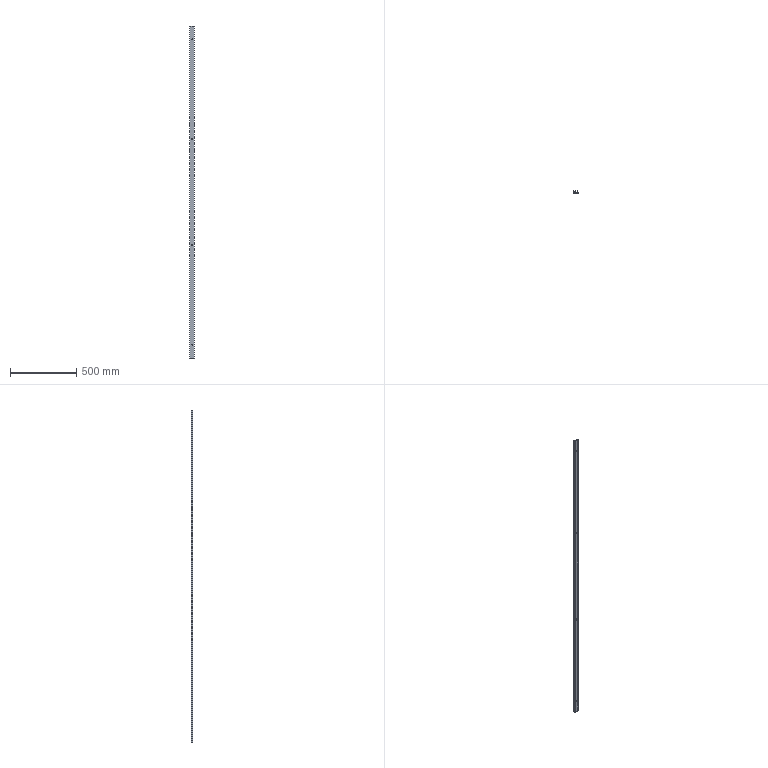Part | SolidWorks | features ICE 2, BaseBody 1, HoleWzd 1, MoveFace 1 | 1 solid | 35 faces | box 33.5 x 13.5 x 2500 mm | volume 468220 mm3 | plane 17 | cylinder 10 | cone 8 | commonest cylinder face diameters 13.44 x4 2 x3 4 x2 1.5 x1
STEP:
#1=CARTESIAN_POINT('',(20.,0.,2303.72));
#2=VERTEX_POINT('',#1);
#3=CARTESIAN_POINT('',(20.,0.,2296.28));
#4=VERTEX_POINT('',#3);
#5=CARTESIAN_POINT('',(20.,0.,2300.));
#6=DIRECTION('',(0.,-1.,0.));
#7=DIRECTION('',(0.,0.,-1.));
#8=AXIS2_PLACEMENT_3D('',#5,#6,#7);
#9=CIRCLE('',#8,3.72);
#10=EDGE_CURVE('',#2,#4,#9,.T.);
#11=ORIENTED_EDGE('',*,*,#10,.T.);
#12=CARTESIAN_POINT('',(20.,3.,2293.28));
#13=VERTEX_POINT('',#12);
#14=CARTESIAN_POINT('',(20.,3.,2293.28));
#15=DIRECTION('',(0.,0.7071,-0.7071));
#16=VECTOR('',#15,1000.);
#17=LINE('',#14,#16);
#18=EDGE_CURVE('',#4,#13,#17,.T.);
#19=ORIENTED_EDGE('',*,*,#18,.T.);
#20=CARTESIAN_POINT('',(20.,3.,2306.72));
#21=VERTEX_POINT('',#20);
#22=CARTESIAN_POINT('',(20.,3.,2300.));
#23=DIRECTION('',(0.,1.,0.));
#24=DIRECTION('',(0.,0.,1.));
#25=AXIS2_PLACEMENT_3D('',#22,#23,#24);
#26=CIRCLE('',#25,6.72);
#27=EDGE_CURVE('',#13,#21,#26,.T.);
#28=ORIENTED_EDGE('',*,*,#27,.T.);
#29=CARTESIAN_POINT('',(20.,3.,2306.72));
#30=DIRECTION('',(0.,0.7071,0.7071));
#31=VECTOR('',#30,1000.);
#32=LINE('',#29,#31);
#33=EDGE_CURVE('',#2,#21,#32,.T.);
#34=ORIENTED_EDGE('',*,*,#33,.F.);
#35=EDGE_LOOP('',(#11,#19,#28,#34));
#36=FACE_OUTER_BOUND('',#35,.T.);
#37=CARTESIAN_POINT('',(20.,3.,2300.));
#38=DIRECTION('',(0.,1.,0.));
#39=DIRECTION('',(0.,0.,1.));
#40=AXIS2_PLACEMENT_3D('',#37,#38,#39);
#41=CONICAL_SURFACE('',#40,6.72,0.7854);
#42=ADVANCED_FACE('',(#36),#41,.F.);
#43=CARTESIAN_POINT('',(20.,0.,3.72));
#44=VERTEX_POINT('',#43);
#45=CARTESIAN_POINT('',(20.,0.,-3.72));
#46=VERTEX_POINT('',#45);
#47=CARTESIAN_POINT('',(20.,0.,0.));
#48=DIRECTION('',(0.,-1.,0.));
#49=DIRECTION('',(0.,0.,-1.));
#50=AXIS2_PLACEMENT_3D('',#47,#48,#49);
#51=CIRCLE('',#50,3.72);
#52=EDGE_CURVE('',#44,#46,#51,.T.);
#53=ORIENTED_EDGE('',*,*,#52,.T.);
#54=CARTESIAN_POINT('',(20.,3.,-6.72));
#55=VERTEX_POINT('',#54);
#56=CARTESIAN_POINT('',(20.,3.,-6.72));
#57=DIRECTION('',(0.,0.7071,-0.7071));
#58=VECTOR('',#57,1000.);
#59=LINE('',#56,#58);
#60=EDGE_CURVE('',#46,#55,#59,.T.);
#61=ORIENTED_EDGE('',*,*,#60,.T.);
#62=CARTESIAN_POINT('',(20.,3.,6.72));
#63=VERTEX_POINT('',#62);
#64=CARTESIAN_POINT('',(20.,3.,0.));
#65=DIRECTION('',(0.,1.,0.));
#66=DIRECTION('',(0.,0.,1.));
#67=AXIS2_PLACEMENT_3D('',#64,#65,#66);
#68=CIRCLE('',#67,6.72);
#69=EDGE_CURVE('',#55,#63,#68,.T.);
#70=ORIENTED_EDGE('',*,*,#69,.T.);
#71=CARTESIAN_POINT('',(20.,3.,6.72));
#72=DIRECTION('',(0.,0.7071,0.7071));
#73=VECTOR('',#72,1000.);
#74=LINE('',#71,#73);
#75=EDGE_CURVE('',#44,#63,#74,.T.);
#76=ORIENTED_EDGE('',*,*,#75,.F.);
#77=EDGE_LOOP('',(#53,#61,#70,#76));
#78=FACE_OUTER_BOUND('',#77,.T.);
#79=CARTESIAN_POINT('',(20.,3.,0.));
#80=DIRECTION('',(0.,1.,0.));
#81=DIRECTION('',(0.,0.,1.));
#82=AXIS2_PLACEMENT_3D('',#79,#80,#81);
#83=CONICAL_SURFACE('',#82,6.72,0.7854);
#84=ADVANCED_FACE('',(#78),#83,.F.);
#85=CARTESIAN_POINT('',(20.,0.,753.72));
#86=VERTEX_POINT('',#85);
#87=CARTESIAN_POINT('',(20.,0.,746.28));
#88=VERTEX_POINT('',#87);
#89=CARTESIAN_POINT('',(20.,0.,750.));
#90=DIRECTION('',(0.,-1.,0.));
#91=DIRECTION('',(0.,0.,-1.));
#92=AXIS2_PLACEMENT_3D('',#89,#90,#91);
#93=CIRCLE('',#92,3.72);
#94=EDGE_CURVE('',#86,#88,#93,.T.);
#95=ORIENTED_EDGE('',*,*,#94,.T.);
#96=CARTESIAN_POINT('',(20.,3.,743.28));
#97=VERTEX_POINT('',#96);
#98=CARTESIAN_POINT('',(20.,3.,743.28));
#99=DIRECTION('',(0.,0.7071,-0.7071));
#100=VECTOR('',#99,1000.);
#101=LINE('',#98,#100);
#102=EDGE_CURVE('',#88,#97,#101,.T.);
#103=ORIENTED_EDGE('',*,*,#102,.T.);
#104=CARTESIAN_POINT('',(20.,3.,756.72));
#105=VERTEX_POINT('',#104);
#106=CARTESIAN_POINT('',(20.,3.,750.));
#107=DIRECTION('',(0.,1.,0.));
#108=DIRECTION('',(0.,0.,1.));
#109=AXIS2_PLACEMENT_3D('',#106,#107,#108);
#110=CIRCLE('',#109,6.72);
#111=EDGE_CURVE('',#97,#105,#110,.T.);
#112=ORIENTED_EDGE('',*,*,#111,.T.);
#113=CARTESIAN_POINT('',(20.,3.,756.72));
#114=DIRECTION('',(0.,0.7071,0.7071));
#115=VECTOR('',#114,1000.);
#116=LINE('',#113,#115);
#117=EDGE_CURVE('',#86,#105,#116,.T.);
#118=ORIENTED_EDGE('',*,*,#117,.F.);
#119=EDGE_LOOP('',(#95,#103,#112,#118));
#120=FACE_OUTER_BOUND('',#119,.T.);
#121=CARTESIAN_POINT('',(20.,3.,750.));
#122=DIRECTION('',(0.,1.,0.));
#123=DIRECTION('',(0.,0.,1.));
#124=AXIS2_PLACEMENT_3D('',#121,#122,#123);
#125=CONICAL_SURFACE('',#124,6.72,0.7854);
#126=ADVANCED_FACE('',(#120),#125,.F.);
#127=CARTESIAN_POINT('',(20.,0.,1553.72));
#128=VERTEX_POINT('',#127);
#129=CARTESIAN_POINT('',(20.,0.,1546.28));
#130=VERTEX_POINT('',#129);
#131=CARTESIAN_POINT('',(20.,0.,1550.));
#132=DIRECTION('',(0.,-1.,0.));
#133=DIRECTION('',(0.,0.,-1.));
#134=AXIS2_PLACEMENT_3D('',#131,#132,#133);
#135=CIRCLE('',#134,3.72);
#136=EDGE_CURVE('',#128,#130,#135,.T.);
#137=ORIENTED_EDGE('',*,*,#136,.T.);
#138=CARTESIAN_POINT('',(20.,3.,1543.28));
#139=VERTEX_POINT('',#138);
#140=CARTESIAN_POINT('',(20.,3.,1543.28));
#141=DIRECTION('',(0.,0.7071,-0.7071));
#142=VECTOR('',#141,1000.);
#143=LINE('',#140,#142);
#144=EDGE_CURVE('',#130,#139,#143,.T.);
#145=ORIENTED_EDGE('',*,*,#144,.T.);
#146=CARTESIAN_POINT('',(20.,3.,1556.72));
#147=VERTEX_POINT('',#146);
#148=CARTESIAN_POINT('',(20.,3.,1550.));
#149=DIRECTION('',(0.,1.,0.));
#150=DIRECTION('',(0.,0.,1.));
#151=AXIS2_PLACEMENT_3D('',#148,#149,#150);
#152=CIRCLE('',#151,6.72);
#153=EDGE_CURVE('',#139,#147,#152,.T.);
#154=ORIENTED_EDGE('',*,*,#153,.T.);
#155=CARTESIAN_POINT('',(20.,3.,1556.72));
#156=DIRECTION('',(0.,0.7071,0.7071));
#157=VECTOR('',#156,1000.);
#158=LINE('',#155,#157);
#159=EDGE_CURVE('',#128,#147,#158,.T.);
#160=ORIENTED_EDGE('',*,*,#159,.F.);
#161=EDGE_LOOP('',(#137,#145,#154,#160));
#162=FACE_OUTER_BOUND('',#161,.T.);
#163=CARTESIAN_POINT('',(20.,3.,1550.));
#164=DIRECTION('',(0.,1.,0.));
#165=DIRECTION('',(0.,0.,1.));
#166=AXIS2_PLACEMENT_3D('',#163,#164,#165);
#167=CONICAL_SURFACE('',#166,6.72,0.7854);
#168=ADVANCED_FACE('',(#162),#167,.F.);
#169=CARTESIAN_POINT('',(24.5,10.5,1545.009));
#170=VERTEX_POINT('',#169);
#171=CARTESIAN_POINT('',(24.5,10.5,754.991));
#172=VERTEX_POINT('',#171);
#173=CARTESIAN_POINT('',(24.5,10.5,-100.));
#174=DIRECTION('',(0.,0.,-1.));
#175=VECTOR('',#174,1000.);
#176=LINE('',#173,#175);
#177=EDGE_CURVE('',#170,#172,#176,.T.);
#178=ORIENTED_EDGE('',*,*,#177,.F.);
#179=CARTESIAN_POINT('',(24.5,10.5,1554.991));
#180=VERTEX_POINT('',#179);
#181=CARTESIAN_POINT('',(24.5,10.5,1545.009));
#182=CARTESIAN_POINT('',(24.5,10.64,1545.009));
#183=CARTESIAN_POINT('',(24.514,10.776,1545.022));
#184=CARTESIAN_POINT('',(24.57,11.042,1545.073));
#185=CARTESIAN_POINT('',(24.611,11.171,1545.111));
#186=CARTESIAN_POINT('',(24.713,11.408,1545.209));
#187=CARTESIAN_POINT('',(24.775,11.519,1545.27));
#188=CARTESIAN_POINT('',(24.908,11.717,1545.409));
#189=CARTESIAN_POINT('',(24.981,11.806,1545.488));
#190=CARTESIAN_POINT('',(25.207,12.042,1545.746));
#191=CARTESIAN_POINT('',(25.363,12.155,1545.942));
#192=CARTESIAN_POINT('',(25.665,12.326,1546.376));
#193=CARTESIAN_POINT('',(25.806,12.38,1546.605));
#194=CARTESIAN_POINT('',(26.061,12.456,1547.084));
#195=CARTESIAN_POINT('',(26.176,12.476,1547.337));
#196=CARTESIAN_POINT('',(26.372,12.498,1547.849));
#197=CARTESIAN_POINT('',(26.454,12.501,1548.109));
#198=CARTESIAN_POINT('',(26.586,12.499,1548.638));
#199=CARTESIAN_POINT('',(26.636,12.496,1548.907));
#200=CARTESIAN_POINT('',(26.703,12.49,1549.453));
#201=CARTESIAN_POINT('',(26.72,12.488,1549.729));
#202=CARTESIAN_POINT('',(26.72,12.488,1550.275));
#203=CARTESIAN_POINT('',(26.703,12.49,1550.547));
#204=CARTESIAN_POINT('',(26.637,12.496,1551.089));
#205=CARTESIAN_POINT('',(26.587,12.499,1551.36));
#206=CARTESIAN_POINT('',(26.387,12.501,1552.161));
#207=CARTESIAN_POINT('',(26.191,12.494,1552.671));
#208=CARTESIAN_POINT('',(25.805,12.38,1553.396));
#209=CARTESIAN_POINT('',(25.663,12.325,1553.627));
#210=CARTESIAN_POINT('',(25.364,12.155,1554.057));
#211=CARTESIAN_POINT('',(25.205,12.039,1554.256));
#212=CARTESIAN_POINT('',(24.981,11.805,1554.512));
#213=CARTESIAN_POINT('',(24.907,11.716,1554.592));
#214=CARTESIAN_POINT('',(24.774,11.518,1554.73));
#215=CARTESIAN_POINT('',(24.714,11.409,1554.79));
#216=CARTESIAN_POINT('',(24.611,11.17,1554.889));
#217=CARTESIAN_POINT('',(24.571,11.044,1554.926));
#218=CARTESIAN_POINT('',(24.515,10.78,1554.977));
#219=CARTESIAN_POINT('',(24.5,10.64,1554.991));
#220=CARTESIAN_POINT('',(24.5,10.5,1554.991));
#221=B_SPLINE_CURVE_WITH_KNOTS('',3,(#181,#182,#183,#184,#185,#186,#187,#188,#189,#190,#191,#192,#193,#194,#195,#196,#197,#198,#199,#200,#201,#202,#203,#204,#205,#206,#207,#208,#209,#210,#211,#212,#213,#214,#215,#216,#217,#218,#219,#220),.UNSPECIFIED.,.F.,.F.,(4,2,2,2,2,2,2,2,2,2,2,2,2,2,2,2,2,2,2,4),(0.,0.0004127,0.0008255,0.001238,0.001651,0.002476,0.003302,0.004127,0.004953,0.005778,0.006604,0.007429,0.008255,0.009906,0.01073,0.01156,0.01197,0.01238,0.01279,0.01321),.UNSPECIFIED.);
#222=EDGE_CURVE('',#170,#180,#221,.T.);
#223=ORIENTED_EDGE('',*,*,#222,.T.);
#224=CARTESIAN_POINT('',(24.5,10.5,2295.009));
#225=VERTEX_POINT('',#224);
#226=CARTESIAN_POINT('',(24.5,10.5,-100.));
#227=DIRECTION('',(0.,0.,-1.));
#228=VECTOR('',#227,1000.);
#229=LINE('',#226,#228);
#230=EDGE_CURVE('',#225,#180,#229,.T.);
#231=ORIENTED_EDGE('',*,*,#230,.F.);
#232=CARTESIAN_POINT('',(24.5,10.5,2304.991));
#233=VERTEX_POINT('',#232);
#234=CARTESIAN_POINT('',(24.5,10.5,2295.009));
#235=CARTESIAN_POINT('',(24.5,10.638,2295.009));
#236=CARTESIAN_POINT('',(24.515,10.777,2295.022));
#237=CARTESIAN_POINT('',(24.57,11.043,2295.073));
#238=CARTESIAN_POINT('',(24.611,11.171,2295.111));
#239=CARTESIAN_POINT('',(24.765,11.529,2295.26));
#240=CARTESIAN_POINT('',(24.907,11.728,2295.403));
#241=CARTESIAN_POINT('',(25.205,12.04,2295.744));
#242=CARTESIAN_POINT('',(25.365,12.156,2295.945));
#243=CARTESIAN_POINT('',(25.663,12.325,2296.373));
#244=CARTESIAN_POINT('',(25.806,12.38,2296.605));
#245=CARTESIAN_POINT('',(26.19,12.494,2297.328));
#246=CARTESIAN_POINT('',(26.387,12.501,2297.839));
#247=CARTESIAN_POINT('',(26.654,12.499,2298.909));
#248=CARTESIAN_POINT('',(26.72,12.488,2299.452));
#249=CARTESIAN_POINT('',(26.72,12.488,2300.277));
#250=CARTESIAN_POINT('',(26.703,12.49,2300.553));
#251=CARTESIAN_POINT('',(26.636,12.496,2301.095));
#252=CARTESIAN_POINT('',(26.586,12.499,2301.362));
#253=CARTESIAN_POINT('',(26.388,12.501,2302.155));
#254=CARTESIAN_POINT('',(26.188,12.493,2302.677));
#255=CARTESIAN_POINT('',(25.805,12.38,2303.396));
#256=CARTESIAN_POINT('',(25.662,12.324,2303.629));
#257=CARTESIAN_POINT('',(25.438,12.197,2303.95));
#258=CARTESIAN_POINT('',(25.362,12.147,2304.053));
#259=CARTESIAN_POINT('',(25.208,12.03,2304.249));
#260=CARTESIAN_POINT('',(25.13,11.961,2304.342));
#261=CARTESIAN_POINT('',(24.98,11.805,2304.513));
#262=CARTESIAN_POINT('',(24.908,11.717,2304.591));
#263=CARTESIAN_POINT('',(24.774,11.518,2304.73));
#264=CARTESIAN_POINT('',(24.714,11.408,2304.79));
#265=CARTESIAN_POINT('',(24.612,11.172,2304.888));
#266=CARTESIAN_POINT('',(24.57,11.043,2304.927));
#267=CARTESIAN_POINT('',(24.515,10.778,2304.978));
#268=CARTESIAN_POINT('',(24.5,10.64,2304.991));
#269=CARTESIAN_POINT('',(24.5,10.5,2304.991));
#270=B_SPLINE_CURVE_WITH_KNOTS('',3,(#234,#235,#236,#237,#238,#239,#240,#241,#242,#243,#244,#245,#246,#247,#248,#249,#250,#251,#252,#253,#254,#255,#256,#257,#258,#259,#260,#261,#262,#263,#264,#265,#266,#267,#268,#269),.UNSPECIFIED.,.F.,.F.,(4,2,2,2,2,2,2,2,2,2,2,2,2,2,2,2,2,4),(0.01321,0.01362,0.01403,0.01486,0.01569,0.01651,0.01816,0.01981,0.02064,0.02146,0.02311,0.02394,0.02435,0.02477,0.02518,0.02559,0.026,0.02642),.UNSPECIFIED.);
#271=EDGE_CURVE('',#225,#233,#270,.T.);
#272=ORIENTED_EDGE('',*,*,#271,.T.);
#273=CARTESIAN_POINT('',(24.5,10.5,2400.));
#274=VERTEX_POINT('',#273);
#275=CARTESIAN_POINT('',(24.5,10.5,-100.));
#276=DIRECTION('',(0.,0.,-1.));
#277=VECTOR('',#276,1000.);
#278=LINE('',#275,#277);
#279=EDGE_CURVE('',#274,#233,#278,.T.);
#280=ORIENTED_EDGE('',*,*,#279,.F.);
#281=CARTESIAN_POINT('',(28.5,10.5,2400.));
#282=VERTEX_POINT('',#281);
#283=CARTESIAN_POINT('',(26.5,10.5,2400.));
#284=DIRECTION('',(0.,0.,1.));
#285=DIRECTION('',(1.,0.,0.));
#286=AXIS2_PLACEMENT_3D('',#283,#284,#285);
#287=CIRCLE('',#286,2.);
#288=EDGE_CURVE('',#282,#274,#287,.T.);
#289=ORIENTED_EDGE('',*,*,#288,.F.);
#290=CARTESIAN_POINT('',(28.5,10.5,-100.));
#291=VERTEX_POINT('',#290);
#292=CARTESIAN_POINT('',(28.5,10.5,-100.));
#293=DIRECTION('',(0.,0.,-1.));
#294=VECTOR('',#293,1000.);
#295=LINE('',#292,#294);
#296=EDGE_CURVE('',#282,#291,#295,.T.);
#297=ORIENTED_EDGE('',*,*,#296,.T.);
#298=CARTESIAN_POINT('',(24.5,10.5,-100.));
#299=VERTEX_POINT('',#298);
#300=CARTESIAN_POINT('',(26.5,10.5,-100.));
#301=DIRECTION('',(0.,0.,1.));
#302=DIRECTION('',(-1.,0.,0.));
#303=AXIS2_PLACEMENT_3D('',#300,#301,#302);
#304=CIRCLE('',#303,2.);
#305=EDGE_CURVE('',#291,#299,#304,.T.);
#306=ORIENTED_EDGE('',*,*,#305,.T.);
#307=CARTESIAN_POINT('',(24.5,10.5,-4.991));
#308=VERTEX_POINT('',#307);
#309=CARTESIAN_POINT('',(24.5,10.5,-100.));
#310=DIRECTION('',(0.,0.,-1.));
#311=VECTOR('',#310,1000.);
#312=LINE('',#309,#311);
#313=EDGE_CURVE('',#308,#299,#312,.T.);
#314=ORIENTED_EDGE('',*,*,#313,.F.);
#315=CARTESIAN_POINT('',(24.5,10.5,4.991));
#316=VERTEX_POINT('',#315);
#317=CARTESIAN_POINT('',(24.5,10.5,-4.991));
#318=CARTESIAN_POINT('',(24.5,10.638,-4.991));
#319=CARTESIAN_POINT('',(24.515,10.777,-4.978));
#320=CARTESIAN_POINT('',(24.57,11.043,-4.927));
#321=CARTESIAN_POINT('',(24.611,11.171,-4.889));
#322=CARTESIAN_POINT('',(24.765,11.529,-4.74));
#323=CARTESIAN_POINT('',(24.907,11.728,-4.597));
#324=CARTESIAN_POINT('',(25.205,12.04,-4.256));
#325=CARTESIAN_POINT('',(25.365,12.156,-4.055));
#326=CARTESIAN_POINT('',(25.663,12.325,-3.627));
#327=CARTESIAN_POINT('',(25.806,12.38,-3.395));
#328=CARTESIAN_POINT('',(26.19,12.494,-2.672));
#329=CARTESIAN_POINT('',(26.387,12.501,-2.161));
#330=CARTESIAN_POINT('',(26.654,12.499,-1.091));
#331=CARTESIAN_POINT('',(26.72,12.488,-0.5481));
#332=CARTESIAN_POINT('',(26.72,12.488,0.2773));
#333=CARTESIAN_POINT('',(26.703,12.49,0.5529));
#334=CARTESIAN_POINT('',(26.636,12.496,1.095));
#335=CARTESIAN_POINT('',(26.586,12.499,1.362));
#336=CARTESIAN_POINT('',(26.388,12.501,2.155));
#337=CARTESIAN_POINT('',(26.188,12.493,2.677));
#338=CARTESIAN_POINT('',(25.805,12.38,3.396));
#339=CARTESIAN_POINT('',(25.662,12.324,3.629));
#340=CARTESIAN_POINT('',(25.438,12.197,3.95));
#341=CARTESIAN_POINT('',(25.362,12.147,4.053));
#342=CARTESIAN_POINT('',(25.208,12.03,4.249));
#343=CARTESIAN_POINT('',(25.13,11.961,4.342));
#344=CARTESIAN_POINT('',(24.98,11.805,4.513));
#345=CARTESIAN_POINT('',(24.908,11.717,4.591));
#346=CARTESIAN_POINT('',(24.774,11.518,4.73));
#347=CARTESIAN_POINT('',(24.714,11.408,4.79));
#348=CARTESIAN_POINT('',(24.612,11.172,4.888));
#349=CARTESIAN_POINT('',(24.57,11.043,4.927));
#350=CARTESIAN_POINT('',(24.515,10.778,4.978));
#351=CARTESIAN_POINT('',(24.5,10.64,4.991));
#352=CARTESIAN_POINT('',(24.5,10.5,4.991));
#353=B_SPLINE_CURVE_WITH_KNOTS('',3,(#317,#318,#319,#320,#321,#322,#323,#324,#325,#326,#327,#328,#329,#330,#331,#332,#333,#334,#335,#336,#337,#338,#339,#340,#341,#342,#343,#344,#345,#346,#347,#348,#349,#350,#351,#352),.UNSPECIFIED.,.F.,.F.,(4,2,2,2,2,2,2,2,2,2,2,2,2,2,2,2,2,4),(0.01321,0.01362,0.01403,0.01486,0.01569,0.01651,0.01816,0.01981,0.02064,0.02146,0.02311,0.02394,0.02435,0.02477,0.02518,0.02559,0.026,0.02642),.UNSPECIFIED.);
#354=EDGE_CURVE('',#308,#316,#353,.T.);
#355=ORIENTED_EDGE('',*,*,#354,.T.);
#356=CARTESIAN_POINT('',(24.5,10.5,745.009));
#357=VERTEX_POINT('',#356);
#358=CARTESIAN_POINT('',(24.5,10.5,-100.));
#359=DIRECTION('',(0.,0.,-1.));
#360=VECTOR('',#359,1000.);
#361=LINE('',#358,#360);
#362=EDGE_CURVE('',#357,#316,#361,.T.);
#363=ORIENTED_EDGE('',*,*,#362,.F.);
#364=CARTESIAN_POINT('',(24.5,10.5,745.009));
#365=CARTESIAN_POINT('',(24.5,10.638,745.009));
#366=CARTESIAN_POINT('',(24.515,10.777,745.022));
#367=CARTESIAN_POINT('',(24.57,11.043,745.073));
#368=CARTESIAN_POINT('',(24.611,11.171,745.111));
#369=CARTESIAN_POINT('',(24.765,11.529,745.26));
#370=CARTESIAN_POINT('',(24.907,11.728,745.403));
#371=CARTESIAN_POINT('',(25.205,12.04,745.744));
#372=CARTESIAN_POINT('',(25.365,12.156,745.945));
#373=CARTESIAN_POINT('',(25.663,12.325,746.373));
#374=CARTESIAN_POINT('',(25.806,12.38,746.605));
#375=CARTESIAN_POINT('',(26.19,12.494,747.328));
#376=CARTESIAN_POINT('',(26.387,12.501,747.839));
#377=CARTESIAN_POINT('',(26.654,12.499,748.909));
#378=CARTESIAN_POINT('',(26.72,12.488,749.452));
#379=CARTESIAN_POINT('',(26.72,12.488,750.277));
#380=CARTESIAN_POINT('',(26.703,12.49,750.553));
#381=CARTESIAN_POINT('',(26.636,12.496,751.095));
#382=CARTESIAN_POINT('',(26.586,12.499,751.362));
#383=CARTESIAN_POINT('',(26.388,12.501,752.155));
#384=CARTESIAN_POINT('',(26.188,12.493,752.677));
#385=CARTESIAN_POINT('',(25.805,12.38,753.396));
#386=CARTESIAN_POINT('',(25.662,12.324,753.629));
#387=CARTESIAN_POINT('',(25.438,12.197,753.95));
#388=CARTESIAN_POINT('',(25.362,12.147,754.053));
#389=CARTESIAN_POINT('',(25.208,12.03,754.249));
#390=CARTESIAN_POINT('',(25.13,11.961,754.342));
#391=CARTESIAN_POINT('',(24.98,11.805,754.513));
#392=CARTESIAN_POINT('',(24.908,11.717,754.591));
#393=CARTESIAN_POINT('',(24.774,11.518,754.73));
#394=CARTESIAN_POINT('',(24.714,11.408,754.79));
#395=CARTESIAN_POINT('',(24.612,11.172,754.888));
#396=CARTESIAN_POINT('',(24.57,11.043,754.927));
#397=CARTESIAN_POINT('',(24.515,10.778,754.978));
#398=CARTESIAN_POINT('',(24.5,10.64,754.991));
#399=CARTESIAN_POINT('',(24.5,10.5,754.991));
#400=B_SPLINE_CURVE_WITH_KNOTS('',3,(#364,#365,#366,#367,#368,#369,#370,#371,#372,#373,#374,#375,#376,#377,#378,#379,#380,#381,#382,#383,#384,#385,#386,#387,#388,#389,#390,#391,#392,#393,#394,#395,#396,#397,#398,#399),.UNSPECIFIED.,.F.,.F.,(4,2,2,2,2,2,2,2,2,2,2,2,2,2,2,2,2,4),(0.01321,0.01362,0.01403,0.01486,0.01569,0.01651,0.01816,0.01981,0.02064,0.02146,0.02311,0.02394,0.02435,0.02477,0.02518,0.02559,0.026,0.02642),.UNSPECIFIED.);
#401=EDGE_CURVE('',#357,#172,#400,.T.);
#402=ORIENTED_EDGE('',*,*,#401,.T.);
#403=EDGE_LOOP('',(#178,#223,#231,#272,#280,#289,#297,#306,#314,#355,#363,#402));
#404=FACE_OUTER_BOUND('',#403,.T.);
#405=CARTESIAN_POINT('',(26.5,10.5,-100.));
#406=DIRECTION('',(0.,0.,-1.));
#407=DIRECTION('',(-1.,0.,0.));
#408=AXIS2_PLACEMENT_3D('',#405,#406,#407);
#409=CYLINDRICAL_SURFACE('',#408,2.);
#410=ADVANCED_FACE('',(#404),#409,.T.);
#411=CARTESIAN_POINT('',(24.5,3.,1545.009));
#412=VERTEX_POINT('',#411);
#413=CARTESIAN_POINT('',(24.5,3.,754.991));
#414=VERTEX_POINT('',#413);
#415=CARTESIAN_POINT('',(24.5,3.,-100.));
#416=DIRECTION('',(0.,0.,-1.));
#417=VECTOR('',#416,1000.);
#418=LINE('',#415,#417);
#419=EDGE_CURVE('',#412,#414,#418,.T.);
#420=ORIENTED_EDGE('',*,*,#419,.F.);
#421=CARTESIAN_POINT('',(24.5,33.,1545.009));
#422=DIRECTION('',(0.,1.,0.));
#423=VECTOR('',#422,1000.);
#424=LINE('',#421,#423);
#425=EDGE_CURVE('',#412,#170,#424,.T.);
#426=ORIENTED_EDGE('',*,*,#425,.T.);
#427=ORIENTED_EDGE('',*,*,#177,.T.);
#428=CARTESIAN_POINT('',(24.5,13.5,754.991));
#429=DIRECTION('',(0.,-1.,0.));
#430=VECTOR('',#429,1000.);
#431=LINE('',#428,#430);
#432=EDGE_CURVE('',#172,#414,#431,.T.);
#433=ORIENTED_EDGE('',*,*,#432,.T.);
#434=EDGE_LOOP('',(#420,#426,#427,#433));
#435=FACE_OUTER_BOUND('',#434,.T.);
#436=CARTESIAN_POINT('',(24.5,10.5,-100.));
#437=DIRECTION('',(-1.,0.,0.));
#438=DIRECTION('',(0.,0.,1.));
#439=AXIS2_PLACEMENT_3D('',#436,#437,#438);
#440=PLANE('',#439);
#441=ADVANCED_FACE('',(#435),#440,.T.);
#442=ORIENTED_EDGE('',*,*,#230,.T.);
#443=CARTESIAN_POINT('',(24.5,3.,1554.991));
#444=VERTEX_POINT('',#443);
#445=CARTESIAN_POINT('',(24.5,33.,1554.991));
#446=DIRECTION('',(0.,-1.,0.));
#447=VECTOR('',#446,1000.);
#448=LINE('',#445,#447);
#449=EDGE_CURVE('',#180,#444,#448,.T.);
#450=ORIENTED_EDGE('',*,*,#449,.T.);
#451=CARTESIAN_POINT('',(24.5,3.,2295.009));
#452=VERTEX_POINT('',#451);
#453=CARTESIAN_POINT('',(24.5,3.,-100.));
#454=DIRECTION('',(0.,0.,-1.));
#455=VECTOR('',#454,1000.);
#456=LINE('',#453,#455);
#457=EDGE_CURVE('',#452,#444,#456,.T.);
#458=ORIENTED_EDGE('',*,*,#457,.F.);
#459=CARTESIAN_POINT('',(24.5,13.5,2295.009));
#460=DIRECTION('',(0.,1.,0.));
#461=VECTOR('',#460,1000.);
#462=LINE('',#459,#461);
#463=EDGE_CURVE('',#452,#225,#462,.T.);
#464=ORIENTED_EDGE('',*,*,#463,.T.);
#465=EDGE_LOOP('',(#442,#450,#458,#464));
#466=FACE_OUTER_BOUND('',#465,.T.);
#467=CARTESIAN_POINT('',(24.5,10.5,-100.));
#468=DIRECTION('',(-1.,0.,0.));
#469=DIRECTION('',(0.,0.,1.));
#470=AXIS2_PLACEMENT_3D('',#467,#468,#469);
#471=PLANE('',#470);
#472=ADVANCED_FACE('',(#466),#471,.T.);
#473=CARTESIAN_POINT('',(24.5,3.,-4.991));
#474=VERTEX_POINT('',#473);
#475=CARTESIAN_POINT('',(24.5,3.,-100.));
#476=VERTEX_POINT('',#475);
#477=CARTESIAN_POINT('',(24.5,3.,-100.));
#478=DIRECTION('',(0.,0.,-1.));
#479=VECTOR('',#478,1000.);
#480=LINE('',#477,#479);
#481=EDGE_CURVE('',#474,#476,#480,.T.);
#482=ORIENTED_EDGE('',*,*,#481,.F.);
#483=CARTESIAN_POINT('',(24.5,13.5,-4.991));
#484=DIRECTION('',(0.,1.,0.));
#485=VECTOR('',#484,1000.);
#486=LINE('',#483,#485);
#487=EDGE_CURVE('',#474,#308,#486,.T.);
#488=ORIENTED_EDGE('',*,*,#487,.T.);
#489=ORIENTED_EDGE('',*,*,#313,.T.);
#490=CARTESIAN_POINT('',(24.5,1.,-100.));
#491=DIRECTION('',(0.,-1.,0.));
#492=VECTOR('',#491,1000.);
#493=LINE('',#490,#492);
#494=EDGE_CURVE('',#299,#476,#493,.T.);
#495=ORIENTED_EDGE('',*,*,#494,.T.);
#496=EDGE_LOOP('',(#482,#488,#489,#495));
#497=FACE_OUTER_BOUND('',#496,.T.);
#498=CARTESIAN_POINT('',(24.5,10.5,-100.));
#499=DIRECTION('',(-1.,0.,0.));
#500=DIRECTION('',(0.,0.,1.));
#501=AXIS2_PLACEMENT_3D('',#498,#499,#500);
#502=PLANE('',#501);
#503=ADVANCED_FACE('',(#497),#502,.T.);
#504=ORIENTED_EDGE('',*,*,#362,.T.);
#505=CARTESIAN_POINT('',(24.5,3.,4.991));
#506=VERTEX_POINT('',#505);
#507=CARTESIAN_POINT('',(24.5,13.5,4.991));
#508=DIRECTION('',(0.,-1.,0.));
#509=VECTOR('',#508,1000.);
#510=LINE('',#507,#509);
#511=EDGE_CURVE('',#316,#506,#510,.T.);
#512=ORIENTED_EDGE('',*,*,#511,.T.);
#513=CARTESIAN_POINT('',(24.5,3.,745.009));
#514=VERTEX_POINT('',#513);
#515=CARTESIAN_POINT('',(24.5,3.,-100.));
#516=DIRECTION('',(0.,0.,-1.));
#517=VECTOR('',#516,1000.);
#518=LINE('',#515,#517);
#519=EDGE_CURVE('',#514,#506,#518,.T.);
#520=ORIENTED_EDGE('',*,*,#519,.F.);
#521=CARTESIAN_POINT('',(24.5,13.5,745.009));
#522=DIRECTION('',(0.,1.,0.));
#523=VECTOR('',#522,1000.);
#524=LINE('',#521,#523);
#525=EDGE_CURVE('',#514,#357,#524,.T.);
#526=ORIENTED_EDGE('',*,*,#525,.T.);
#527=EDGE_LOOP('',(#504,#512,#520,#526));
#528=FACE_OUTER_BOUND('',#527,.T.);
#529=CARTESIAN_POINT('',(24.5,10.5,-100.));
#530=DIRECTION('',(-1.,0.,0.));
#531=DIRECTION('',(0.,0.,1.));
#532=AXIS2_PLACEMENT_3D('',#529,#530,#531);
#533=PLANE('',#532);
#534=ADVANCED_FACE('',(#528),#533,.T.);
#535=ORIENTED_EDGE('',*,*,#279,.T.);
#536=CARTESIAN_POINT('',(24.5,3.,2304.991));
#537=VERTEX_POINT('',#536);
#538=CARTESIAN_POINT('',(24.5,13.5,2304.991));
#539=DIRECTION('',(0.,-1.,0.));
#540=VECTOR('',#539,1000.);
#541=LINE('',#538,#540);
#542=EDGE_CURVE('',#233,#537,#541,.T.);
#543=ORIENTED_EDGE('',*,*,#542,.T.);
#544=CARTESIAN_POINT('',(24.5,3.,2400.));
#545=VERTEX_POINT('',#544);
#546=CARTESIAN_POINT('',(24.5,3.,-100.));
#547=DIRECTION('',(0.,0.,-1.));
#548=VECTOR('',#547,1000.);
#549=LINE('',#546,#548);
#550=EDGE_CURVE('',#545,#537,#549,.T.);
#551=ORIENTED_EDGE('',*,*,#550,.F.);
#552=CARTESIAN_POINT('',(24.5,1.,2400.));
#553=DIRECTION('',(0.,-1.,0.));
#554=VECTOR('',#553,1000.);
#555=LINE('',#552,#554);
#556=EDGE_CURVE('',#274,#545,#555,.T.);
#557=ORIENTED_EDGE('',*,*,#556,.F.);
#558=EDGE_LOOP('',(#535,#543,#551,#557));
#559=FACE_OUTER_BOUND('',#558,.T.);
#560=CARTESIAN_POINT('',(24.5,10.5,-100.));
#561=DIRECTION('',(-1.,0.,0.));
#562=DIRECTION('',(0.,0.,1.));
#563=AXIS2_PLACEMENT_3D('',#560,#561,#562);
#564=PLANE('',#563);
#565=ADVANCED_FACE('',(#559),#564,.T.);
#566=ORIENTED_EDGE('',*,*,#10,.F.);
#567=CARTESIAN_POINT('',(20.,0.,2300.));
#568=DIRECTION('',(0.,-1.,0.));
#569=DIRECTION('',(0.,0.,-1.));
#570=AXIS2_PLACEMENT_3D('',#567,#568,#569);
#571=CIRCLE('',#570,3.72);
#572=EDGE_CURVE('',#4,#2,#571,.T.);
#573=ORIENTED_EDGE('',*,*,#572,.F.);
#574=EDGE_LOOP('',(#566,#573));
#575=FACE_BOUND('',#574,.T.);
#576=ORIENTED_EDGE('',*,*,#94,.F.);
#577=CARTESIAN_POINT('',(20.,0.,750.));
#578=DIRECTION('',(0.,-1.,0.));
#579=DIRECTION('',(0.,0.,-1.));
#580=AXIS2_PLACEMENT_3D('',#577,#578,#579);
#581=CIRCLE('',#580,3.72);
#582=EDGE_CURVE('',#88,#86,#581,.T.);
#583=ORIENTED_EDGE('',*,*,#582,.F.);
#584=EDGE_LOOP('',(#576,#583));
#585=FACE_BOUND('',#584,.T.);
#586=ORIENTED_EDGE('',*,*,#136,.F.);
#587=CARTESIAN_POINT('',(20.,0.,1550.));
#588=DIRECTION('',(0.,-1.,0.));
#589=DIRECTION('',(0.,0.,-1.));
#590=AXIS2_PLACEMENT_3D('',#587,#588,#589);
#591=CIRCLE('',#590,3.72);
#592=EDGE_CURVE('',#130,#128,#591,.T.);
#593=ORIENTED_EDGE('',*,*,#592,.F.);
#594=EDGE_LOOP('',(#586,#593));
#595=FACE_BOUND('',#594,.T.);
#596=CARTESIAN_POINT('',(1.,0.,-100.));
#597=VERTEX_POINT('',#596);
#598=CARTESIAN_POINT('',(32.5,0.,-100.));
#599=VERTEX_POINT('',#598);
#600=CARTESIAN_POINT('',(1.,0.,-100.));
#601=DIRECTION('',(1.,0.,0.));
#602=VECTOR('',#601,1000.);
#603=LINE('',#600,#602);
#604=EDGE_CURVE('',#597,#599,#603,.T.);
#605=ORIENTED_EDGE('',*,*,#604,.T.);
#606=CARTESIAN_POINT('',(32.5,0.,2400.));
#607=VERTEX_POINT('',#606);
#608=CARTESIAN_POINT('',(32.5,0.,-100.));
#609=DIRECTION('',(0.,0.,1.));
#610=VECTOR('',#609,1000.);
#611=LINE('',#608,#610);
#612=EDGE_CURVE('',#599,#607,#611,.T.);
#613=ORIENTED_EDGE('',*,*,#612,.T.);
#614=CARTESIAN_POINT('',(1.,0.,2400.));
#615=VERTEX_POINT('',#614);
#616=CARTESIAN_POINT('',(1.,0.,2400.));
#617=DIRECTION('',(-1.,0.,0.));
#618=VECTOR('',#617,1000.);
#619=LINE('',#616,#618);
#620=EDGE_CURVE('',#607,#615,#619,.T.);
#621=ORIENTED_EDGE('',*,*,#620,.T.);
#622=CARTESIAN_POINT('',(1.,0.,-100.));
#623=DIRECTION('',(0.,0.,-1.));
#624=VECTOR('',#623,1000.);
#625=LINE('',#622,#624);
#626=EDGE_CURVE('',#615,#597,#625,.T.);
#627=ORIENTED_EDGE('',*,*,#626,.T.);
#628=EDGE_LOOP('',(#605,#613,#621,#627));
#629=FACE_OUTER_BOUND('',#628,.T.);
#630=ORIENTED_EDGE('',*,*,#52,.F.);
#631=CARTESIAN_POINT('',(20.,0.,0.));
#632=DIRECTION('',(0.,-1.,0.));
#633=DIRECTION('',(0.,0.,-1.));
#634=AXIS2_PLACEMENT_3D('',#631,#632,#633);
#635=CIRCLE('',#634,3.72);
#636=EDGE_CURVE('',#46,#44,#635,.T.);
#637=ORIENTED_EDGE('',*,*,#636,.F.);
#638=EDGE_LOOP('',(#630,#637));
#639=FACE_BOUND('',#638,.T.);
#640=CARTESIAN_POINT('',(1.,0.,-100.));
#641=DIRECTION('',(0.,-1.,0.));
#642=DIRECTION('',(0.,0.,-1.));
#643=AXIS2_PLACEMENT_3D('',#640,#641,#642);
#644=PLANE('',#643);
#645=ADVANCED_FACE('',(#575,#585,#595,#629,#639),#644,.T.);
#646=CARTESIAN_POINT('',(33.5,1.,-100.));
#647=VERTEX_POINT('',#646);
#648=CARTESIAN_POINT('',(32.5,1.,-100.));
#649=DIRECTION('',(0.,0.,1.));
#650=DIRECTION('',(-1.,0.,0.));
#651=AXIS2_PLACEMENT_3D('',#648,#649,#650);
#652=CIRCLE('',#651,1.);
#653=EDGE_CURVE('',#599,#647,#652,.T.);
#654=ORIENTED_EDGE('',*,*,#653,.T.);
#655=CARTESIAN_POINT('',(33.5,1.,2400.));
#656=VERTEX_POINT('',#655);
#657=CARTESIAN_POINT('',(33.5,1.,-100.));
#658=DIRECTION('',(0.,0.,1.));
#659=VECTOR('',#658,1000.);
#660=LINE('',#657,#659);
#661=EDGE_CURVE('',#647,#656,#660,.T.);
#662=ORIENTED_EDGE('',*,*,#661,.T.);
#663=CARTESIAN_POINT('',(32.5,1.,2400.));
#664=DIRECTION('',(0.,0.,-1.));
#665=DIRECTION('',(1.,0.,0.));
#666=AXIS2_PLACEMENT_3D('',#663,#664,#665);
#667=CIRCLE('',#666,1.);
#668=EDGE_CURVE('',#656,#607,#667,.T.);
#669=ORIENTED_EDGE('',*,*,#668,.T.);
#670=ORIENTED_EDGE('',*,*,#612,.F.);
#671=EDGE_LOOP('',(#654,#662,#669,#670));
#672=FACE_OUTER_BOUND('',#671,.T.);
#673=CARTESIAN_POINT('',(32.5,1.,-100.));
#674=DIRECTION('',(0.,0.,-1.));
#675=DIRECTION('',(-1.,0.,0.));
#676=AXIS2_PLACEMENT_3D('',#673,#674,#675);
#677=CYLINDRICAL_SURFACE('',#676,1.);
#678=ADVANCED_FACE('',(#672),#677,.T.);
#679=CARTESIAN_POINT('',(1.5,12.75,-100.));
#680=VERTEX_POINT('',#679);
#681=CARTESIAN_POINT('',(0.,12.75,-100.));
#682=VERTEX_POINT('',#681);
#683=CARTESIAN_POINT('',(0.75,12.75,-100.));
#684=DIRECTION('',(0.,0.,1.));
#685=DIRECTION('',(-1.,0.,0.));
#686=AXIS2_PLACEMENT_3D('',#683,#684,#685);
#687=CIRCLE('',#686,0.75);
#688=EDGE_CURVE('',#680,#682,#687,.T.);
#689=ORIENTED_EDGE('',*,*,#688,.F.);
#690=CARTESIAN_POINT('',(1.5,3.,-100.));
#691=VERTEX_POINT('',#690);
#692=CARTESIAN_POINT('',(1.5,1.,-100.));
#693=DIRECTION('',(0.,1.,0.));
#694=VECTOR('',#693,1000.);
#695=LINE('',#692,#694);
#696=EDGE_CURVE('',#691,#680,#695,.T.);
#697=ORIENTED_EDGE('',*,*,#696,.F.);
#698=CARTESIAN_POINT('',(8.5,3.,-100.));
#699=VERTEX_POINT('',#698);
#700=CARTESIAN_POINT('',(1.,3.,-100.));
#701=DIRECTION('',(-1.,0.,0.));
#702=VECTOR('',#701,1000.);
#703=LINE('',#700,#702);
#704=EDGE_CURVE('',#699,#691,#703,.T.);
#705=ORIENTED_EDGE('',*,*,#704,.F.);
#706=CARTESIAN_POINT('',(8.5,10.5,-100.));
#707=VERTEX_POINT('',#706);
#708=CARTESIAN_POINT('',(8.5,1.,-100.));
#709=DIRECTION('',(0.,-1.,0.));
#710=VECTOR('',#709,1000.);
#711=LINE('',#708,#710);
#712=EDGE_CURVE('',#707,#699,#711,.T.);
#713=ORIENTED_EDGE('',*,*,#712,.F.);
#714=CARTESIAN_POINT('',(12.5,10.5,-100.));
#715=VERTEX_POINT('',#714);
#716=CARTESIAN_POINT('',(10.5,10.5,-100.));
#717=DIRECTION('',(0.,0.,1.));
#718=DIRECTION('',(-1.,0.,0.));
#719=AXIS2_PLACEMENT_3D('',#716,#717,#718);
#720=CIRCLE('',#719,2.);
#721=EDGE_CURVE('',#715,#707,#720,.T.);
#722=ORIENTED_EDGE('',*,*,#721,.F.);
#723=CARTESIAN_POINT('',(12.5,3.,-100.));
#724=VERTEX_POINT('',#723);
#725=CARTESIAN_POINT('',(12.5,1.,-100.));
#726=DIRECTION('',(0.,1.,0.));
#727=VECTOR('',#726,1000.);
#728=LINE('',#725,#727);
#729=EDGE_CURVE('',#724,#715,#728,.T.);
#730=ORIENTED_EDGE('',*,*,#729,.F.);
#731=CARTESIAN_POINT('',(1.,3.,-100.));
#732=DIRECTION('',(-1.,0.,0.));
#733=VECTOR('',#732,1000.);
#734=LINE('',#731,#733);
#735=EDGE_CURVE('',#476,#724,#734,.T.);
#736=ORIENTED_EDGE('',*,*,#735,.F.);
#737=ORIENTED_EDGE('',*,*,#494,.F.);
#738=ORIENTED_EDGE('',*,*,#305,.F.);
#739=CARTESIAN_POINT('',(28.5,3.,-100.));
#740=VERTEX_POINT('',#739);
#741=CARTESIAN_POINT('',(28.5,1.,-100.));
#742=DIRECTION('',(0.,1.,0.));
#743=VECTOR('',#742,1000.);
#744=LINE('',#741,#743);
#745=EDGE_CURVE('',#740,#291,#744,.T.);
#746=ORIENTED_EDGE('',*,*,#745,.F.);
#747=CARTESIAN_POINT('',(32.5,3.,-100.));
#748=VERTEX_POINT('',#747);
#749=CARTESIAN_POINT('',(1.,3.,-100.));
#750=DIRECTION('',(-1.,0.,0.));
#751=VECTOR('',#750,1000.);
#752=LINE('',#749,#751);
#753=EDGE_CURVE('',#748,#740,#752,.T.);
#754=ORIENTED_EDGE('',*,*,#753,.F.);
#755=CARTESIAN_POINT('',(33.5,2.,-100.));
#756=VERTEX_POINT('',#755);
#757=CARTESIAN_POINT('',(32.5,2.,-100.));
#758=DIRECTION('',(0.,0.,1.));
#759=DIRECTION('',(-1.,0.,0.));
#760=AXIS2_PLACEMENT_3D('',#757,#758,#759);
#761=CIRCLE('',#760,1.);
#762=EDGE_CURVE('',#756,#748,#761,.T.);
#763=ORIENTED_EDGE('',*,*,#762,.F.);
#764=CARTESIAN_POINT('',(33.5,1.,-100.));
#765=DIRECTION('',(0.,1.,0.));
#766=VECTOR('',#765,1000.);
#767=LINE('',#764,#766);
#768=EDGE_CURVE('',#647,#756,#767,.T.);
#769=ORIENTED_EDGE('',*,*,#768,.F.);
#770=ORIENTED_EDGE('',*,*,#653,.F.);
#771=ORIENTED_EDGE('',*,*,#604,.F.);
#772=CARTESIAN_POINT('',(0.,1.,-100.));
#773=VERTEX_POINT('',#772);
#774=CARTESIAN_POINT('',(1.,1.,-100.));
#775=DIRECTION('',(0.,0.,1.));
#776=DIRECTION('',(-1.,0.,0.));
#777=AXIS2_PLACEMENT_3D('',#774,#775,#776);
#778=CIRCLE('',#777,1.);
#779=EDGE_CURVE('',#773,#597,#778,.T.);
#780=ORIENTED_EDGE('',*,*,#779,.F.);
#781=CARTESIAN_POINT('',(0.,1.,-100.));
#782=DIRECTION('',(0.,-1.,0.));
#783=VECTOR('',#782,1000.);
#784=LINE('',#781,#783);
#785=EDGE_CURVE('',#682,#773,#784,.T.);
#786=ORIENTED_EDGE('',*,*,#785,.F.);
#787=EDGE_LOOP('',(#689,#697,#705,#713,#722,#730,#736,#737,#738,#746,#754,#763,#769,#770,#771,#780,#786));
#788=FACE_OUTER_BOUND('',#787,.T.);
#789=CARTESIAN_POINT('',(1.,1.,-100.));
#790=DIRECTION('',(0.,0.,1.));
#791=DIRECTION('',(1.,0.,0.));
#792=AXIS2_PLACEMENT_3D('',#789,#790,#791);
#793=PLANE('',#792);
#794=ADVANCED_FACE('',(#788),#793,.F.);
#795=ORIENTED_EDGE('',*,*,#779,.T.);
#796=ORIENTED_EDGE('',*,*,#626,.F.);
#797=CARTESIAN_POINT('',(0.,1.,2400.));
#798=VERTEX_POINT('',#797);
#799=CARTESIAN_POINT('',(1.,1.,2400.));
#800=DIRECTION('',(0.,0.,-1.));
#801=DIRECTION('',(1.,0.,0.));
#802=AXIS2_PLACEMENT_3D('',#799,#800,#801);
#803=CIRCLE('',#802,1.);
#804=EDGE_CURVE('',#615,#798,#803,.T.);
#805=ORIENTED_EDGE('',*,*,#804,.T.);
#806=CARTESIAN_POINT('',(0.,1.,-100.));
#807=DIRECTION('',(0.,0.,-1.));
#808=VECTOR('',#807,1000.);
#809=LINE('',#806,#808);
#810=EDGE_CURVE('',#798,#773,#809,.T.);
#811=ORIENTED_EDGE('',*,*,#810,.T.);
#812=EDGE_LOOP('',(#795,#796,#805,#811));
#813=FACE_OUTER_BOUND('',#812,.T.);
#814=CARTESIAN_POINT('',(1.,1.,-100.));
#815=DIRECTION('',(0.,0.,-1.));
#816=DIRECTION('',(-1.,0.,0.));
#817=AXIS2_PLACEMENT_3D('',#814,#815,#816);
#818=CYLINDRICAL_SURFACE('',#817,1.);
#819=ADVANCED_FACE('',(#813),#818,.T.);
#820=CARTESIAN_POINT('',(1.5,3.,2400.));
#821=VERTEX_POINT('',#820);
#822=CARTESIAN_POINT('',(1.5,12.75,2400.));
#823=VERTEX_POINT('',#822);
#824=CARTESIAN_POINT('',(1.5,1.,2400.));
#825=DIRECTION('',(0.,1.,0.));
#826=VECTOR('',#825,1000.);
#827=LINE('',#824,#826);
#828=EDGE_CURVE('',#821,#823,#827,.T.);
#829=ORIENTED_EDGE('',*,*,#828,.T.);
#830=CARTESIAN_POINT('',(0.,12.75,2400.));
#831=VERTEX_POINT('',#830);
#832=CARTESIAN_POINT('',(0.75,12.75,2400.));
#833=DIRECTION('',(0.,0.,1.));
#834=DIRECTION('',(1.,0.,0.));
#835=AXIS2_PLACEMENT_3D('',#832,#833,#834);
#836=CIRCLE('',#835,0.75);
#837=EDGE_CURVE('',#823,#831,#836,.T.);
#838=ORIENTED_EDGE('',*,*,#837,.T.);
#839=CARTESIAN_POINT('',(0.,1.,2400.));
#840=DIRECTION('',(0.,-1.,0.));
#841=VECTOR('',#840,1000.);
#842=LINE('',#839,#841);
#843=EDGE_CURVE('',#831,#798,#842,.T.);
#844=ORIENTED_EDGE('',*,*,#843,.T.);
#845=ORIENTED_EDGE('',*,*,#804,.F.);
#846=ORIENTED_EDGE('',*,*,#620,.F.);
#847=ORIENTED_EDGE('',*,*,#668,.F.);
#848=CARTESIAN_POINT('',(33.5,2.,2400.));
#849=VERTEX_POINT('',#848);
#850=CARTESIAN_POINT('',(33.5,1.,2400.));
#851=DIRECTION('',(0.,1.,0.));
#852=VECTOR('',#851,1000.);
#853=LINE('',#850,#852);
#854=EDGE_CURVE('',#656,#849,#853,.T.);
#855=ORIENTED_EDGE('',*,*,#854,.T.);
#856=CARTESIAN_POINT('',(32.5,3.,2400.));
#857=VERTEX_POINT('',#856);
#858=CARTESIAN_POINT('',(32.5,2.,2400.));
#859=DIRECTION('',(0.,0.,-1.));
#860=DIRECTION('',(1.,0.,0.));
#861=AXIS2_PLACEMENT_3D('',#858,#859,#860);
#862=CIRCLE('',#861,1.);
#863=EDGE_CURVE('',#857,#849,#862,.T.);
#864=ORIENTED_EDGE('',*,*,#863,.F.);
#865=CARTESIAN_POINT('',(28.5,3.,2400.));
#866=VERTEX_POINT('',#865);
#867=CARTESIAN_POINT('',(1.,3.,2400.));
#868=DIRECTION('',(-1.,0.,0.));
#869=VECTOR('',#868,1000.);
#870=LINE('',#867,#869);
#871=EDGE_CURVE('',#857,#866,#870,.T.);
#872=ORIENTED_EDGE('',*,*,#871,.T.);
#873=CARTESIAN_POINT('',(28.5,1.,2400.));
#874=DIRECTION('',(0.,1.,0.));
#875=VECTOR('',#874,1000.);
#876=LINE('',#873,#875);
#877=EDGE_CURVE('',#866,#282,#876,.T.);
#878=ORIENTED_EDGE('',*,*,#877,.T.);
#879=ORIENTED_EDGE('',*,*,#288,.T.);
#880=ORIENTED_EDGE('',*,*,#556,.T.);
#881=CARTESIAN_POINT('',(12.5,3.,2400.));
#882=VERTEX_POINT('',#881);
#883=CARTESIAN_POINT('',(1.,3.,2400.));
#884=DIRECTION('',(-1.,0.,0.));
#885=VECTOR('',#884,1000.);
#886=LINE('',#883,#885);
#887=EDGE_CURVE('',#545,#882,#886,.T.);
#888=ORIENTED_EDGE('',*,*,#887,.T.);
#889=CARTESIAN_POINT('',(12.5,10.5,2400.));
#890=VERTEX_POINT('',#889);
#891=CARTESIAN_POINT('',(12.5,1.,2400.));
#892=DIRECTION('',(0.,1.,0.));
#893=VECTOR('',#892,1000.);
#894=LINE('',#891,#893);
#895=EDGE_CURVE('',#882,#890,#894,.T.);
#896=ORIENTED_EDGE('',*,*,#895,.T.);
#897=CARTESIAN_POINT('',(8.5,10.5,2400.));
#898=VERTEX_POINT('',#897);
#899=CARTESIAN_POINT('',(10.5,10.5,2400.));
#900=DIRECTION('',(0.,0.,1.));
#901=DIRECTION('',(1.,0.,0.));
#902=AXIS2_PLACEMENT_3D('',#899,#900,#901);
#903=CIRCLE('',#902,2.);
#904=EDGE_CURVE('',#890,#898,#903,.T.);
#905=ORIENTED_EDGE('',*,*,#904,.T.);
#906=CARTESIAN_POINT('',(8.5,3.,2400.));
#907=VERTEX_POINT('',#906);
#908=CARTESIAN_POINT('',(8.5,1.,2400.));
#909=DIRECTION('',(0.,-1.,0.));
#910=VECTOR('',#909,1000.);
#911=LINE('',#908,#910);
#912=EDGE_CURVE('',#898,#907,#911,.T.);
#913=ORIENTED_EDGE('',*,*,#912,.T.);
#914=CARTESIAN_POINT('',(1.,3.,2400.));
#915=DIRECTION('',(-1.,0.,0.));
#916=VECTOR('',#915,1000.);
#917=LINE('',#914,#916);
#918=EDGE_CURVE('',#907,#821,#917,.T.);
#919=ORIENTED_EDGE('',*,*,#918,.T.);
#920=EDGE_LOOP('',(#829,#838,#844,#845,#846,#847,#855,#864,#872,#878,#879,#880,#888,#896,#905,#913,#919));
#921=FACE_OUTER_BOUND('',#920,.T.);
#922=CARTESIAN_POINT('',(1.,1.,2400.));
#923=DIRECTION('',(0.,0.,1.));
#924=DIRECTION('',(1.,0.,0.));
#925=AXIS2_PLACEMENT_3D('',#922,#923,#924);
#926=PLANE('',#925);
#927=ADVANCED_FACE('',(#921),#926,.T.);
#928=ORIENTED_EDGE('',*,*,#768,.T.);
#929=CARTESIAN_POINT('',(33.5,2.,-100.));
#930=DIRECTION('',(0.,0.,1.));
#931=VECTOR('',#930,1000.);
#932=LINE('',#929,#931);
#933=EDGE_CURVE('',#756,#849,#932,.T.);
#934=ORIENTED_EDGE('',*,*,#933,.T.);
#935=ORIENTED_EDGE('',*,*,#854,.F.);
#936=ORIENTED_EDGE('',*,*,#661,.F.);
#937=EDGE_LOOP('',(#928,#934,#935,#936));
#938=FACE_OUTER_BOUND('',#937,.T.);
#939=CARTESIAN_POINT('',(33.5,1.,-100.));
#940=DIRECTION('',(1.,0.,0.));
#941=DIRECTION('',(0.,0.,-1.));
#942=AXIS2_PLACEMENT_3D('',#939,#940,#941);
#943=PLANE('',#942);
#944=ADVANCED_FACE('',(#938),#943,.T.);
#945=ORIENTED_EDGE('',*,*,#785,.T.);
#946=ORIENTED_EDGE('',*,*,#810,.F.);
#947=ORIENTED_EDGE('',*,*,#843,.F.);
#948=CARTESIAN_POINT('',(0.,12.75,-100.));
#949=DIRECTION('',(0.,0.,-1.));
#950=VECTOR('',#949,1000.);
#951=LINE('',#948,#950);
#952=EDGE_CURVE('',#831,#682,#951,.T.);
#953=ORIENTED_EDGE('',*,*,#952,.T.);
#954=EDGE_LOOP('',(#945,#946,#947,#953));
#955=FACE_OUTER_BOUND('',#954,.T.);
#956=CARTESIAN_POINT('',(0.,12.75,-100.));
#957=DIRECTION('',(-1.,0.,0.));
#958=DIRECTION('',(0.,0.,1.));
#959=AXIS2_PLACEMENT_3D('',#956,#957,#958);
#960=PLANE('',#959);
#961=ADVANCED_FACE('',(#955),#960,.T.);
#962=ORIENTED_EDGE('',*,*,#688,.T.);
#963=ORIENTED_EDGE('',*,*,#952,.F.);
#964=ORIENTED_EDGE('',*,*,#837,.F.);
#965=CARTESIAN_POINT('',(1.5,12.75,-100.));
#966=DIRECTION('',(0.,0.,-1.));
#967=VECTOR('',#966,1000.);
#968=LINE('',#965,#967);
#969=EDGE_CURVE('',#823,#680,#968,.T.);
#970=ORIENTED_EDGE('',*,*,#969,.T.);
#971=EDGE_LOOP('',(#962,#963,#964,#970));
#972=FACE_OUTER_BOUND('',#971,.T.);
#973=CARTESIAN_POINT('',(0.75,12.75,-100.));
#974=DIRECTION('',(0.,0.,-1.));
#975=DIRECTION('',(-1.,0.,0.));
#976=AXIS2_PLACEMENT_3D('',#973,#974,#975);
#977=CYLINDRICAL_SURFACE('',#976,0.75);
#978=ADVANCED_FACE('',(#972),#977,.T.);
#979=ORIENTED_EDGE('',*,*,#696,.T.);
#980=ORIENTED_EDGE('',*,*,#969,.F.);
#981=ORIENTED_EDGE('',*,*,#828,.F.);
#982=CARTESIAN_POINT('',(1.5,3.,-100.));
#983=DIRECTION('',(0.,0.,-1.));
#984=VECTOR('',#983,1000.);
#985=LINE('',#982,#984);
#986=EDGE_CURVE('',#821,#691,#985,.T.);
#987=ORIENTED_EDGE('',*,*,#986,.T.);
#988=EDGE_LOOP('',(#979,#980,#981,#987));
#989=FACE_OUTER_BOUND('',#988,.T.);
#990=CARTESIAN_POINT('',(1.5,3.,-100.));
#991=DIRECTION('',(1.,0.,0.));
#992=DIRECTION('',(0.,0.,-1.));
#993=AXIS2_PLACEMENT_3D('',#990,#991,#992);
#994=PLANE('',#993);
#995=ADVANCED_FACE('',(#989),#994,.T.);
#996=ORIENTED_EDGE('',*,*,#704,.T.);
#997=ORIENTED_EDGE('',*,*,#986,.F.);
#998=ORIENTED_EDGE('',*,*,#918,.F.);
#999=CARTESIAN_POINT('',(8.5,3.,-100.));
#1000=DIRECTION('',(0.,0.,-1.));
#1001=VECTOR('',#1000,1000.);
#1002=LINE('',#999,#1001);
#1003=EDGE_CURVE('',#907,#699,#1002,.T.);
#1004=ORIENTED_EDGE('',*,*,#1003,.T.);
#1005=EDGE_LOOP('',(#996,#997,#998,#1004));
#1006=FACE_OUTER_BOUND('',#1005,.T.);
#1007=CARTESIAN_POINT('',(8.5,3.,-100.));
#1008=DIRECTION('',(0.,1.,0.));
#1009=DIRECTION('',(0.,0.,1.));
#1010=AXIS2_PLACEMENT_3D('',#1007,#1008,#1009);
#1011=PLANE('',#1010);
#1012=ADVANCED_FACE('',(#1006),#1011,.T.);
#1013=ORIENTED_EDGE('',*,*,#712,.T.);
#1014=ORIENTED_EDGE('',*,*,#1003,.F.);
#1015=ORIENTED_EDGE('',*,*,#912,.F.);
#1016=CARTESIAN_POINT('',(8.5,10.5,-100.));
#1017=DIRECTION('',(0.,0.,-1.));
#1018=VECTOR('',#1017,1000.);
#1019=LINE('',#1016,#1018);
#1020=EDGE_CURVE('',#898,#707,#1019,.T.);
#1021=ORIENTED_EDGE('',*,*,#1020,.T.);
#1022=EDGE_LOOP('',(#1013,#1014,#1015,#1021));
#1023=FACE_OUTER_BOUND('',#1022,.T.);
#1024=CARTESIAN_POINT('',(8.5,10.5,-100.));
#1025=DIRECTION('',(-1.,0.,0.));
#1026=DIRECTION('',(0.,0.,1.));
#1027=AXIS2_PLACEMENT_3D('',#1024,#1025,#1026);
#1028=PLANE('',#1027);
#1029=ADVANCED_FACE('',(#1023),#1028,.T.);
#1030=ORIENTED_EDGE('',*,*,#721,.T.);
#1031=ORIENTED_EDGE('',*,*,#1020,.F.);
#1032=ORIENTED_EDGE('',*,*,#904,.F.);
#1033=CARTESIAN_POINT('',(12.5,10.5,-100.));
#1034=DIRECTION('',(0.,0.,-1.));
#1035=VECTOR('',#1034,1000.);
#1036=LINE('',#1033,#1035);
#1037=EDGE_CURVE('',#890,#715,#1036,.T.);
#1038=ORIENTED_EDGE('',*,*,#1037,.T.);
#1039=EDGE_LOOP('',(#1030,#1031,#1032,#1038));
#1040=FACE_OUTER_BOUND('',#1039,.T.);
#1041=CARTESIAN_POINT('',(10.5,10.5,-100.));
#1042=DIRECTION('',(0.,0.,-1.));
#1043=DIRECTION('',(-1.,0.,0.));
#1044=AXIS2_PLACEMENT_3D('',#1041,#1042,#1043);
#1045=CYLINDRICAL_SURFACE('',#1044,2.);
#1046=ADVANCED_FACE('',(#1040),#1045,.T.);
#1047=ORIENTED_EDGE('',*,*,#729,.T.);
#1048=ORIENTED_EDGE('',*,*,#1037,.F.);
#1049=ORIENTED_EDGE('',*,*,#895,.F.);
#1050=CARTESIAN_POINT('',(12.5,3.,-100.));
#1051=DIRECTION('',(0.,0.,-1.));
#1052=VECTOR('',#1051,1000.);
#1053=LINE('',#1050,#1052);
#1054=EDGE_CURVE('',#882,#724,#1053,.T.);
#1055=ORIENTED_EDGE('',*,*,#1054,.T.);
#1056=EDGE_LOOP('',(#1047,#1048,#1049,#1055));
#1057=FACE_OUTER_BOUND('',#1056,.T.);
#1058=CARTESIAN_POINT('',(12.5,3.,-100.));
#1059=DIRECTION('',(1.,0.,0.));
#1060=DIRECTION('',(0.,0.,-1.));
#1061=AXIS2_PLACEMENT_3D('',#1058,#1059,#1060);
#1062=PLANE('',#1061);
#1063=ADVANCED_FACE('',(#1057),#1062,.T.);
#1064=CARTESIAN_POINT('',(20.,3.,2300.));
#1065=DIRECTION('',(0.,1.,0.));
#1066=DIRECTION('',(0.,0.,1.));
#1067=AXIS2_PLACEMENT_3D('',#1064,#1065,#1066);
#1068=CIRCLE('',#1067,6.72);
#1069=EDGE_CURVE('',#452,#13,#1068,.T.);
#1070=ORIENTED_EDGE('',*,*,#1069,.F.);
#1071=ORIENTED_EDGE('',*,*,#457,.T.);
#1072=CARTESIAN_POINT('',(20.,3.,1550.));
#1073=DIRECTION('',(0.,1.,0.));
#1074=DIRECTION('',(0.,0.,1.));
#1075=AXIS2_PLACEMENT_3D('',#1072,#1073,#1074);
#1076=CIRCLE('',#1075,6.72);
#1077=EDGE_CURVE('',#147,#444,#1076,.T.);
#1078=ORIENTED_EDGE('',*,*,#1077,.F.);
#1079=ORIENTED_EDGE('',*,*,#153,.F.);
#1080=CARTESIAN_POINT('',(20.,3.,1550.));
#1081=DIRECTION('',(0.,1.,0.));
#1082=DIRECTION('',(0.,0.,1.));
#1083=AXIS2_PLACEMENT_3D('',#1080,#1081,#1082);
#1084=CIRCLE('',#1083,6.72);
#1085=EDGE_CURVE('',#412,#139,#1084,.T.);
#1086=ORIENTED_EDGE('',*,*,#1085,.F.);
#1087=ORIENTED_EDGE('',*,*,#419,.T.);
#1088=CARTESIAN_POINT('',(20.,3.,750.));
#1089=DIRECTION('',(0.,1.,0.));
#1090=DIRECTION('',(0.,0.,1.));
#1091=AXIS2_PLACEMENT_3D('',#1088,#1089,#1090);
#1092=CIRCLE('',#1091,6.72);
#1093=EDGE_CURVE('',#105,#414,#1092,.T.);
#1094=ORIENTED_EDGE('',*,*,#1093,.F.);
#1095=ORIENTED_EDGE('',*,*,#111,.F.);
#1096=CARTESIAN_POINT('',(20.,3.,750.));
#1097=DIRECTION('',(0.,1.,0.));
#1098=DIRECTION('',(0.,0.,1.));
#1099=AXIS2_PLACEMENT_3D('',#1096,#1097,#1098);
#1100=CIRCLE('',#1099,6.72);
#1101=EDGE_CURVE('',#514,#97,#1100,.T.);
#1102=ORIENTED_EDGE('',*,*,#1101,.F.);
#1103=ORIENTED_EDGE('',*,*,#519,.T.);
#1104=CARTESIAN_POINT('',(20.,3.,0.));
#1105=DIRECTION('',(0.,1.,0.));
#1106=DIRECTION('',(0.,0.,1.));
#1107=AXIS2_PLACEMENT_3D('',#1104,#1105,#1106);
#1108=CIRCLE('',#1107,6.72);
#1109=EDGE_CURVE('',#63,#506,#1108,.T.);
#1110=ORIENTED_EDGE('',*,*,#1109,.F.);
#1111=ORIENTED_EDGE('',*,*,#69,.F.);
#1112=CARTESIAN_POINT('',(20.,3.,0.));
#1113=DIRECTION('',(0.,1.,0.));
#1114=DIRECTION('',(0.,0.,1.));
#1115=AXIS2_PLACEMENT_3D('',#1112,#1113,#1114);
#1116=CIRCLE('',#1115,6.72);
#1117=EDGE_CURVE('',#474,#55,#1116,.T.);
#1118=ORIENTED_EDGE('',*,*,#1117,.F.);
#1119=ORIENTED_EDGE('',*,*,#481,.T.);
#1120=ORIENTED_EDGE('',*,*,#735,.T.);
#1121=ORIENTED_EDGE('',*,*,#1054,.F.);
#1122=ORIENTED_EDGE('',*,*,#887,.F.);
#1123=ORIENTED_EDGE('',*,*,#550,.T.);
#1124=CARTESIAN_POINT('',(20.,3.,2300.));
#1125=DIRECTION('',(0.,1.,0.));
#1126=DIRECTION('',(0.,0.,1.));
#1127=AXIS2_PLACEMENT_3D('',#1124,#1125,#1126);
#1128=CIRCLE('',#1127,6.72);
#1129=EDGE_CURVE('',#21,#537,#1128,.T.);
#1130=ORIENTED_EDGE('',*,*,#1129,.F.);
#1131=ORIENTED_EDGE('',*,*,#27,.F.);
#1132=EDGE_LOOP('',(#1070,#1071,#1078,#1079,#1086,#1087,#1094,#1095,#1102,#1103,#1110,#1111,#1118,#1119,#1120,#1121,#1122,#1123,#1130,#1131));
#1133=FACE_OUTER_BOUND('',#1132,.T.);
#1134=CARTESIAN_POINT('',(24.5,3.,-100.));
#1135=DIRECTION('',(0.,1.,0.));
#1136=DIRECTION('',(0.,0.,1.));
#1137=AXIS2_PLACEMENT_3D('',#1134,#1135,#1136);
#1138=PLANE('',#1137);
#1139=ADVANCED_FACE('',(#1133),#1138,.T.);
#1140=ORIENTED_EDGE('',*,*,#745,.T.);
#1141=ORIENTED_EDGE('',*,*,#296,.F.);
#1142=ORIENTED_EDGE('',*,*,#877,.F.);
#1143=CARTESIAN_POINT('',(28.5,3.,-100.));
#1144=DIRECTION('',(0.,0.,-1.));
#1145=VECTOR('',#1144,1000.);
#1146=LINE('',#1143,#1145);
#1147=EDGE_CURVE('',#866,#740,#1146,.T.);
#1148=ORIENTED_EDGE('',*,*,#1147,.T.);
#1149=EDGE_LOOP('',(#1140,#1141,#1142,#1148));
#1150=FACE_OUTER_BOUND('',#1149,.T.);
#1151=CARTESIAN_POINT('',(28.5,3.,-100.));
#1152=DIRECTION('',(1.,0.,0.));
#1153=DIRECTION('',(0.,0.,-1.));
#1154=AXIS2_PLACEMENT_3D('',#1151,#1152,#1153);
#1155=PLANE('',#1154);
#1156=ADVANCED_FACE('',(#1150),#1155,.T.);
#1157=ORIENTED_EDGE('',*,*,#753,.T.);
#1158=ORIENTED_EDGE('',*,*,#1147,.F.);
#1159=ORIENTED_EDGE('',*,*,#871,.F.);
#1160=CARTESIAN_POINT('',(32.5,3.,-100.));
#1161=DIRECTION('',(0.,0.,-1.));
#1162=VECTOR('',#1161,1000.);
#1163=LINE('',#1160,#1162);
#1164=EDGE_CURVE('',#857,#748,#1163,.T.);
#1165=ORIENTED_EDGE('',*,*,#1164,.T.);
#1166=EDGE_LOOP('',(#1157,#1158,#1159,#1165));
#1167=FACE_OUTER_BOUND('',#1166,.T.);
#1168=CARTESIAN_POINT('',(32.5,3.,-100.));
#1169=DIRECTION('',(0.,1.,0.));
#1170=DIRECTION('',(0.,0.,1.));
#1171=AXIS2_PLACEMENT_3D('',#1168,#1169,#1170);
#1172=PLANE('',#1171);
#1173=ADVANCED_FACE('',(#1167),#1172,.T.);
#1174=ORIENTED_EDGE('',*,*,#762,.T.);
#1175=ORIENTED_EDGE('',*,*,#1164,.F.);
#1176=ORIENTED_EDGE('',*,*,#863,.T.);
#1177=ORIENTED_EDGE('',*,*,#933,.F.);
#1178=EDGE_LOOP('',(#1174,#1175,#1176,#1177));
#1179=FACE_OUTER_BOUND('',#1178,.T.);
#1180=CARTESIAN_POINT('',(32.5,2.,-100.));
#1181=DIRECTION('',(0.,0.,-1.));
#1182=DIRECTION('',(-1.,0.,0.));
#1183=AXIS2_PLACEMENT_3D('',#1180,#1181,#1182);
#1184=CYLINDRICAL_SURFACE('',#1183,1.);
#1185=ADVANCED_FACE('',(#1179),#1184,.T.);
#1186=ORIENTED_EDGE('',*,*,#144,.F.);
#1187=ORIENTED_EDGE('',*,*,#592,.T.);
#1188=ORIENTED_EDGE('',*,*,#159,.T.);
#1189=ORIENTED_EDGE('',*,*,#1077,.T.);
#1190=CARTESIAN_POINT('',(20.,3.,1550.));
#1191=DIRECTION('',(0.,1.,0.));
#1192=DIRECTION('',(0.,0.,1.));
#1193=AXIS2_PLACEMENT_3D('',#1190,#1191,#1192);
#1194=CIRCLE('',#1193,6.72);
#1195=EDGE_CURVE('',#444,#412,#1194,.T.);
#1196=ORIENTED_EDGE('',*,*,#1195,.T.);
#1197=ORIENTED_EDGE('',*,*,#1085,.T.);
#1198=EDGE_LOOP('',(#1186,#1187,#1188,#1189,#1196,#1197));
#1199=FACE_OUTER_BOUND('',#1198,.T.);
#1200=CARTESIAN_POINT('',(20.,3.,1550.));
#1201=DIRECTION('',(0.,1.,0.));
#1202=DIRECTION('',(0.,0.,1.));
#1203=AXIS2_PLACEMENT_3D('',#1200,#1201,#1202);
#1204=CONICAL_SURFACE('',#1203,6.72,0.7854);
#1205=ADVANCED_FACE('',(#1199),#1204,.F.);
#1206=ORIENTED_EDGE('',*,*,#102,.F.);
#1207=ORIENTED_EDGE('',*,*,#582,.T.);
#1208=ORIENTED_EDGE('',*,*,#117,.T.);
#1209=ORIENTED_EDGE('',*,*,#1093,.T.);
#1210=CARTESIAN_POINT('',(20.,3.,750.));
#1211=DIRECTION('',(0.,1.,0.));
#1212=DIRECTION('',(0.,0.,1.));
#1213=AXIS2_PLACEMENT_3D('',#1210,#1211,#1212);
#1214=CIRCLE('',#1213,6.72);
#1215=EDGE_CURVE('',#414,#514,#1214,.T.);
#1216=ORIENTED_EDGE('',*,*,#1215,.T.);
#1217=ORIENTED_EDGE('',*,*,#1101,.T.);
#1218=EDGE_LOOP('',(#1206,#1207,#1208,#1209,#1216,#1217));
#1219=FACE_OUTER_BOUND('',#1218,.T.);
#1220=CARTESIAN_POINT('',(20.,3.,750.));
#1221=DIRECTION('',(0.,1.,0.));
#1222=DIRECTION('',(0.,0.,1.));
#1223=AXIS2_PLACEMENT_3D('',#1220,#1221,#1222);
#1224=CONICAL_SURFACE('',#1223,6.72,0.7854);
#1225=ADVANCED_FACE('',(#1219),#1224,.F.);
#1226=ORIENTED_EDGE('',*,*,#60,.F.);
#1227=ORIENTED_EDGE('',*,*,#636,.T.);
#1228=ORIENTED_EDGE('',*,*,#75,.T.);
#1229=ORIENTED_EDGE('',*,*,#1109,.T.);
#1230=CARTESIAN_POINT('',(20.,3.,0.));
#1231=DIRECTION('',(0.,1.,0.));
#1232=DIRECTION('',(0.,0.,1.));
#1233=AXIS2_PLACEMENT_3D('',#1230,#1231,#1232);
#1234=CIRCLE('',#1233,6.72);
#1235=EDGE_CURVE('',#506,#474,#1234,.T.);
#1236=ORIENTED_EDGE('',*,*,#1235,.T.);
#1237=ORIENTED_EDGE('',*,*,#1117,.T.);
#1238=EDGE_LOOP('',(#1226,#1227,#1228,#1229,#1236,#1237));
#1239=FACE_OUTER_BOUND('',#1238,.T.);
#1240=CARTESIAN_POINT('',(20.,3.,0.));
#1241=DIRECTION('',(0.,1.,0.));
#1242=DIRECTION('',(0.,0.,1.));
#1243=AXIS2_PLACEMENT_3D('',#1240,#1241,#1242);
#1244=CONICAL_SURFACE('',#1243,6.72,0.7854);
#1245=ADVANCED_FACE('',(#1239),#1244,.F.);
#1246=ORIENTED_EDGE('',*,*,#18,.F.);
#1247=ORIENTED_EDGE('',*,*,#572,.T.);
#1248=ORIENTED_EDGE('',*,*,#33,.T.);
#1249=ORIENTED_EDGE('',*,*,#1129,.T.);
#1250=CARTESIAN_POINT('',(20.,3.,2300.));
#1251=DIRECTION('',(0.,1.,0.));
#1252=DIRECTION('',(0.,0.,1.));
#1253=AXIS2_PLACEMENT_3D('',#1250,#1251,#1252);
#1254=CIRCLE('',#1253,6.72);
#1255=EDGE_CURVE('',#537,#452,#1254,.T.);
#1256=ORIENTED_EDGE('',*,*,#1255,.T.);
#1257=ORIENTED_EDGE('',*,*,#1069,.T.);
#1258=EDGE_LOOP('',(#1246,#1247,#1248,#1249,#1256,#1257));
#1259=FACE_OUTER_BOUND('',#1258,.T.);
#1260=CARTESIAN_POINT('',(20.,3.,2300.));
#1261=DIRECTION('',(0.,1.,0.));
#1262=DIRECTION('',(0.,0.,1.));
#1263=AXIS2_PLACEMENT_3D('',#1260,#1261,#1262);
#1264=CONICAL_SURFACE('',#1263,6.72,0.7854);
#1265=ADVANCED_FACE('',(#1259),#1264,.F.);
#1266=ORIENTED_EDGE('',*,*,#1255,.F.);
#1267=ORIENTED_EDGE('',*,*,#542,.F.);
#1268=ORIENTED_EDGE('',*,*,#271,.F.);
#1269=ORIENTED_EDGE('',*,*,#463,.F.);
#1270=EDGE_LOOP('',(#1266,#1267,#1268,#1269));
#1271=FACE_OUTER_BOUND('',#1270,.T.);
#1272=CARTESIAN_POINT('',(20.,13.5,2300.));
#1273=DIRECTION('',(0.,-1.,0.));
#1274=DIRECTION('',(0.,0.,-1.));
#1275=AXIS2_PLACEMENT_3D('',#1272,#1273,#1274);
#1276=CYLINDRICAL_SURFACE('',#1275,6.72);
#1277=ADVANCED_FACE('',(#1271),#1276,.F.);
#1278=ORIENTED_EDGE('',*,*,#1215,.F.);
#1279=ORIENTED_EDGE('',*,*,#432,.F.);
#1280=ORIENTED_EDGE('',*,*,#401,.F.);
#1281=ORIENTED_EDGE('',*,*,#525,.F.);
#1282=EDGE_LOOP('',(#1278,#1279,#1280,#1281));
#1283=FACE_OUTER_BOUND('',#1282,.T.);
#1284=CARTESIAN_POINT('',(20.,13.5,750.));
#1285=DIRECTION('',(0.,-1.,0.));
#1286=DIRECTION('',(0.,0.,-1.));
#1287=AXIS2_PLACEMENT_3D('',#1284,#1285,#1286);
#1288=CYLINDRICAL_SURFACE('',#1287,6.72);
#1289=ADVANCED_FACE('',(#1283),#1288,.F.);
#1290=ORIENTED_EDGE('',*,*,#1235,.F.);
#1291=ORIENTED_EDGE('',*,*,#511,.F.);
#1292=ORIENTED_EDGE('',*,*,#354,.F.);
#1293=ORIENTED_EDGE('',*,*,#487,.F.);
#1294=EDGE_LOOP('',(#1290,#1291,#1292,#1293));
#1295=FACE_OUTER_BOUND('',#1294,.T.);
#1296=CARTESIAN_POINT('',(20.,13.5,0.));
#1297=DIRECTION('',(0.,-1.,0.));
#1298=DIRECTION('',(0.,0.,-1.));
#1299=AXIS2_PLACEMENT_3D('',#1296,#1297,#1298);
#1300=CYLINDRICAL_SURFACE('',#1299,6.72);
#1301=ADVANCED_FACE('',(#1295),#1300,.F.);
#1302=ORIENTED_EDGE('',*,*,#1195,.F.);
#1303=ORIENTED_EDGE('',*,*,#449,.F.);
#1304=ORIENTED_EDGE('',*,*,#222,.F.);
#1305=ORIENTED_EDGE('',*,*,#425,.F.);
#1306=EDGE_LOOP('',(#1302,#1303,#1304,#1305));
#1307=FACE_OUTER_BOUND('',#1306,.T.);
#1308=CARTESIAN_POINT('',(20.,33.,1550.));
#1309=DIRECTION('',(0.,-1.,0.));
#1310=DIRECTION('',(0.,0.,-1.));
#1311=AXIS2_PLACEMENT_3D('',#1308,#1309,#1310);
#1312=CYLINDRICAL_SURFACE('',#1311,6.72);
#1313=ADVANCED_FACE('',(#1307),#1312,.F.);
#1314=CLOSED_SHELL('',(#42,#84,#126,#168,#410,#441,#472,#503,#534,#565,#645,#678,#794,#819,#927,#944,#961,#978,#995,#1012,#1029,#1046,#1063,#1139,#1156,#1173,#1185,#1205,#1225,#1245,#1265,#1277,#1289,#1301,#1313));
#1315=MANIFOLD_SOLID_BREP('',#1314);
#1316=CARTESIAN_POINT('',(0.,0.,0.));
#1317=DIRECTION('',(0.,0.,1.));
#1318=DIRECTION('',(1.,0.,0.));
#1319=AXIS2_PLACEMENT_3D('',#1316,#1317,#1318);
#1320=(LENGTH_UNIT()NAMED_UNIT(*)SI_UNIT(.MILLI.,.METRE.));
#1321=UNCERTAINTY_MEASURE_WITH_UNIT(LENGTH_MEASURE(0.00001),#1320,'','');
#1322=(NAMED_UNIT(*)PLANE_ANGLE_UNIT()SI_UNIT($,.RADIAN.));
#1323=(NAMED_UNIT(*)SI_UNIT($,.STERADIAN.)SOLID_ANGLE_UNIT());
#1324=(GEOMETRIC_REPRESENTATION_CONTEXT(3)GLOBAL_UNCERTAINTY_ASSIGNED_CONTEXT((#1321))GLOBAL_UNIT_ASSIGNED_CONTEXT((#1320,#1322,#1323))REPRESENTATION_CONTEXT('',''));
#1325=ADVANCED_BREP_SHAPE_REPRESENTATION('',(#1315,#1319),#1324);